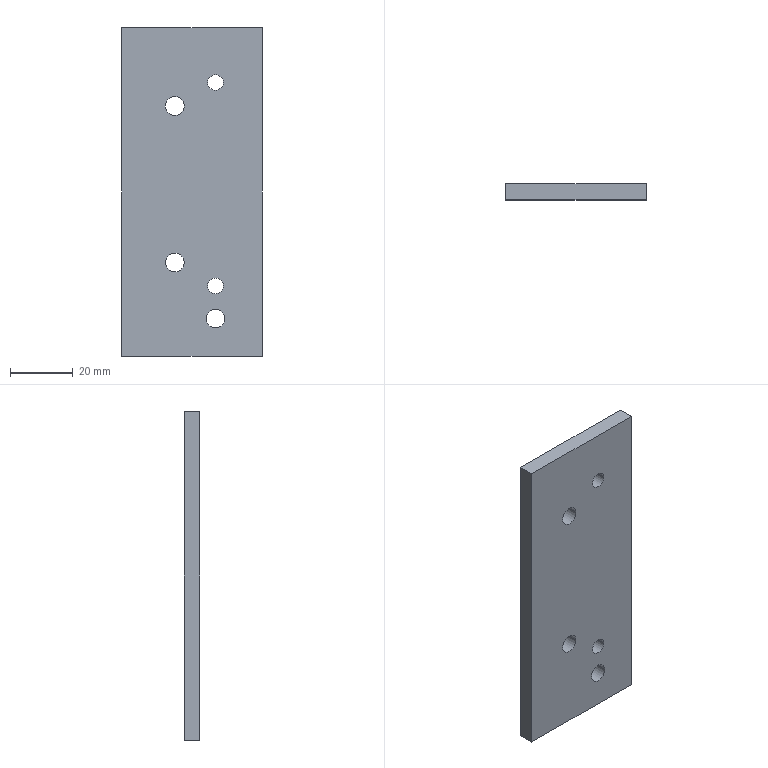Part | STEP file | 1 solid | 16 faces | box 45 x 5 x 105 mm | volume 23005 mm3 | cylinder 10 | plane 6 | commonest cylinder face diameters 6 x6 5 x4
STEP:
#1=CARTESIAN_POINT('',(0.,0.,0.));
#2=DIRECTION('',(0.,0.,1.));
#3=DIRECTION('',(1.,0.,0.));
#4=AXIS2_PLACEMENT_3D('',#1,#2,#3);
#5=CARTESIAN_POINT('',(10.,0.,-30.));
#6=VERTEX_POINT('',#5);
#7=CARTESIAN_POINT('',(10.,5.,-30.));
#8=VERTEX_POINT('',#7);
#9=CARTESIAN_POINT('',(10.,5.,-30.));
#10=DIRECTION('',(0.,1.,0.));
#11=VECTOR('',#10,1.);
#12=LINE('',#9,#11);
#13=CARTESIAN_POINT('',(7.5,5.,-30.));
#14=DIRECTION('',(0.,1.,0.));
#15=DIRECTION('',(1.,0.,0.));
#16=AXIS2_PLACEMENT_3D('',#13,#14,#15);
#17=CYLINDRICAL_SURFACE('',#16,2.5);
#18=CARTESIAN_POINT('',(6.283,0.));
#19=DIRECTION('',(0.,1.));
#20=VECTOR('',#19,1.);
#21=LINE('',#18,#20);
#22=(GEOMETRIC_REPRESENTATION_CONTEXT(2)PARAMETRIC_REPRESENTATION_CONTEXT()REPRESENTATION_CONTEXT('',''));
#23=DEFINITIONAL_REPRESENTATION('',(#21),#22);
#24=PCURVE('',#17,#23);
#25=CARTESIAN_POINT('',(7.5,5.,-30.));
#26=DIRECTION('',(0.,1.,0.));
#27=DIRECTION('',(1.,0.,0.));
#28=AXIS2_PLACEMENT_3D('',#25,#26,#27);
#29=CYLINDRICAL_SURFACE('',#28,2.5);
#30=CARTESIAN_POINT('',(0.,0.));
#31=DIRECTION('',(0.,1.));
#32=VECTOR('',#31,1.);
#33=LINE('',#30,#32);
#34=(GEOMETRIC_REPRESENTATION_CONTEXT(2)PARAMETRIC_REPRESENTATION_CONTEXT()REPRESENTATION_CONTEXT('',''));
#35=DEFINITIONAL_REPRESENTATION('',(#33),#34);
#36=PCURVE('',#29,#35);
#37=SURFACE_CURVE('',#12,(#24,#36),.PCURVE_S1.);
#38=EDGE_CURVE('',#6,#8,#37,.T.);
#39=ORIENTED_EDGE('',*,*,#38,.T.);
#40=CARTESIAN_POINT('',(5.,5.,-30.));
#41=VERTEX_POINT('',#40);
#42=CARTESIAN_POINT('',(7.5,5.,-30.));
#43=DIRECTION('',(0.,1.,0.));
#44=DIRECTION('',(1.,0.,0.));
#45=AXIS2_PLACEMENT_3D('',#42,#43,#44);
#46=CIRCLE('',#45,2.5);
#47=CARTESIAN_POINT('',(0.,0.));
#48=DIRECTION('',(1.,0.));
#49=VECTOR('',#48,1.);
#50=LINE('',#47,#49);
#51=(GEOMETRIC_REPRESENTATION_CONTEXT(2)PARAMETRIC_REPRESENTATION_CONTEXT()REPRESENTATION_CONTEXT('',''));
#52=DEFINITIONAL_REPRESENTATION('',(#50),#51);
#53=PCURVE('',#17,#52);
#54=CARTESIAN_POINT('',(0.,5.,0.));
#55=DIRECTION('',(0.,1.,0.));
#56=DIRECTION('',(0.,0.,1.));
#57=AXIS2_PLACEMENT_3D('',#54,#55,#56);
#58=PLANE('',#57);
#59=CARTESIAN_POINT('',(-30.,7.5));
#60=DIRECTION('',(0.,1.));
#61=AXIS2_PLACEMENT_2D('',#59,#60);
#62=CIRCLE('',#61,2.5);
#63=(GEOMETRIC_REPRESENTATION_CONTEXT(2)PARAMETRIC_REPRESENTATION_CONTEXT()REPRESENTATION_CONTEXT('',''));
#64=DEFINITIONAL_REPRESENTATION('',(#62),#63);
#65=PCURVE('',#58,#64);
#66=SURFACE_CURVE('',#46,(#53,#65),.PCURVE_S1.);
#67=EDGE_CURVE('',#41,#8,#66,.T.);
#68=ORIENTED_EDGE('',*,*,#67,.F.);
#69=CARTESIAN_POINT('',(5.,0.,-30.));
#70=VERTEX_POINT('',#69);
#71=CARTESIAN_POINT('',(5.,5.,-30.));
#72=DIRECTION('',(0.,1.,0.));
#73=VECTOR('',#72,1.);
#74=LINE('',#71,#73);
#75=CARTESIAN_POINT('',(3.142,0.));
#76=DIRECTION('',(0.,1.));
#77=VECTOR('',#76,1.);
#78=LINE('',#75,#77);
#79=(GEOMETRIC_REPRESENTATION_CONTEXT(2)PARAMETRIC_REPRESENTATION_CONTEXT()REPRESENTATION_CONTEXT('',''));
#80=DEFINITIONAL_REPRESENTATION('',(#78),#79);
#81=PCURVE('',#17,#80);
#82=CARTESIAN_POINT('',(3.142,0.));
#83=DIRECTION('',(0.,1.));
#84=VECTOR('',#83,1.);
#85=LINE('',#82,#84);
#86=(GEOMETRIC_REPRESENTATION_CONTEXT(2)PARAMETRIC_REPRESENTATION_CONTEXT()REPRESENTATION_CONTEXT('',''));
#87=DEFINITIONAL_REPRESENTATION('',(#85),#86);
#88=PCURVE('',#29,#87);
#89=SURFACE_CURVE('',#74,(#81,#88),.PCURVE_S1.);
#90=EDGE_CURVE('',#70,#41,#89,.T.);
#91=ORIENTED_EDGE('',*,*,#90,.F.);
#92=CARTESIAN_POINT('',(7.5,0.,-30.));
#93=DIRECTION('',(0.,1.,0.));
#94=DIRECTION('',(0.,0.,1.));
#95=AXIS2_PLACEMENT_3D('',#92,#93,#94);
#96=CIRCLE('',#95,2.5);
#97=CARTESIAN_POINT('',(-1.571,-5.));
#98=DIRECTION('',(1.,0.));
#99=VECTOR('',#98,1.);
#100=LINE('',#97,#99);
#101=(GEOMETRIC_REPRESENTATION_CONTEXT(2)PARAMETRIC_REPRESENTATION_CONTEXT()REPRESENTATION_CONTEXT('',''));
#102=DEFINITIONAL_REPRESENTATION('',(#100),#101);
#103=PCURVE('',#17,#102);
#104=CARTESIAN_POINT('',(0.,0.,0.));
#105=DIRECTION('',(0.,1.,0.));
#106=DIRECTION('',(0.,0.,1.));
#107=AXIS2_PLACEMENT_3D('',#104,#105,#106);
#108=PLANE('',#107);
#109=CARTESIAN_POINT('',(-30.,7.5));
#110=DIRECTION('',(1.,0.));
#111=AXIS2_PLACEMENT_2D('',#109,#110);
#112=CIRCLE('',#111,2.5);
#113=(GEOMETRIC_REPRESENTATION_CONTEXT(2)PARAMETRIC_REPRESENTATION_CONTEXT()REPRESENTATION_CONTEXT('',''));
#114=DEFINITIONAL_REPRESENTATION('',(#112),#113);
#115=PCURVE('',#108,#114);
#116=SURFACE_CURVE('',#96,(#103,#115),.PCURVE_S1.);
#117=EDGE_CURVE('',#70,#6,#116,.T.);
#118=ORIENTED_EDGE('',*,*,#117,.T.);
#119=EDGE_LOOP('',(#39,#68,#91,#118));
#120=FACE_BOUND('',#119,.F.);
#121=ADVANCED_FACE('',(#120),#17,.F.);
#122=CARTESIAN_POINT('',(10.,0.,35.));
#123=VERTEX_POINT('',#122);
#124=CARTESIAN_POINT('',(10.,5.,35.));
#125=VERTEX_POINT('',#124);
#126=CARTESIAN_POINT('',(10.,5.,35.));
#127=DIRECTION('',(0.,1.,0.));
#128=VECTOR('',#127,1.);
#129=LINE('',#126,#128);
#130=CARTESIAN_POINT('',(7.5,5.,35.));
#131=DIRECTION('',(0.,1.,0.));
#132=DIRECTION('',(1.,0.,0.));
#133=AXIS2_PLACEMENT_3D('',#130,#131,#132);
#134=CYLINDRICAL_SURFACE('',#133,2.5);
#135=CARTESIAN_POINT('',(6.283,0.));
#136=DIRECTION('',(0.,1.));
#137=VECTOR('',#136,1.);
#138=LINE('',#135,#137);
#139=(GEOMETRIC_REPRESENTATION_CONTEXT(2)PARAMETRIC_REPRESENTATION_CONTEXT()REPRESENTATION_CONTEXT('',''));
#140=DEFINITIONAL_REPRESENTATION('',(#138),#139);
#141=PCURVE('',#134,#140);
#142=CARTESIAN_POINT('',(7.5,5.,35.));
#143=DIRECTION('',(0.,1.,0.));
#144=DIRECTION('',(1.,0.,0.));
#145=AXIS2_PLACEMENT_3D('',#142,#143,#144);
#146=CYLINDRICAL_SURFACE('',#145,2.5);
#147=CARTESIAN_POINT('',(0.,0.));
#148=DIRECTION('',(0.,1.));
#149=VECTOR('',#148,1.);
#150=LINE('',#147,#149);
#151=(GEOMETRIC_REPRESENTATION_CONTEXT(2)PARAMETRIC_REPRESENTATION_CONTEXT()REPRESENTATION_CONTEXT('',''));
#152=DEFINITIONAL_REPRESENTATION('',(#150),#151);
#153=PCURVE('',#146,#152);
#154=SURFACE_CURVE('',#129,(#141,#153),.PCURVE_S1.);
#155=EDGE_CURVE('',#123,#125,#154,.T.);
#156=ORIENTED_EDGE('',*,*,#155,.T.);
#157=CARTESIAN_POINT('',(5.,5.,35.));
#158=VERTEX_POINT('',#157);
#159=CARTESIAN_POINT('',(7.5,5.,35.));
#160=DIRECTION('',(0.,1.,0.));
#161=DIRECTION('',(1.,0.,0.));
#162=AXIS2_PLACEMENT_3D('',#159,#160,#161);
#163=CIRCLE('',#162,2.5);
#164=CARTESIAN_POINT('',(0.,0.));
#165=DIRECTION('',(1.,0.));
#166=VECTOR('',#165,1.);
#167=LINE('',#164,#166);
#168=(GEOMETRIC_REPRESENTATION_CONTEXT(2)PARAMETRIC_REPRESENTATION_CONTEXT()REPRESENTATION_CONTEXT('',''));
#169=DEFINITIONAL_REPRESENTATION('',(#167),#168);
#170=PCURVE('',#134,#169);
#171=CARTESIAN_POINT('',(35.,7.5));
#172=DIRECTION('',(0.,1.));
#173=AXIS2_PLACEMENT_2D('',#171,#172);
#174=CIRCLE('',#173,2.5);
#175=(GEOMETRIC_REPRESENTATION_CONTEXT(2)PARAMETRIC_REPRESENTATION_CONTEXT()REPRESENTATION_CONTEXT('',''));
#176=DEFINITIONAL_REPRESENTATION('',(#174),#175);
#177=PCURVE('',#58,#176);
#178=SURFACE_CURVE('',#163,(#170,#177),.PCURVE_S1.);
#179=EDGE_CURVE('',#158,#125,#178,.T.);
#180=ORIENTED_EDGE('',*,*,#179,.F.);
#181=CARTESIAN_POINT('',(5.,0.,35.));
#182=VERTEX_POINT('',#181);
#183=CARTESIAN_POINT('',(5.,5.,35.));
#184=DIRECTION('',(0.,1.,0.));
#185=VECTOR('',#184,1.);
#186=LINE('',#183,#185);
#187=CARTESIAN_POINT('',(3.142,0.));
#188=DIRECTION('',(0.,1.));
#189=VECTOR('',#188,1.);
#190=LINE('',#187,#189);
#191=(GEOMETRIC_REPRESENTATION_CONTEXT(2)PARAMETRIC_REPRESENTATION_CONTEXT()REPRESENTATION_CONTEXT('',''));
#192=DEFINITIONAL_REPRESENTATION('',(#190),#191);
#193=PCURVE('',#134,#192);
#194=CARTESIAN_POINT('',(3.142,0.));
#195=DIRECTION('',(0.,1.));
#196=VECTOR('',#195,1.);
#197=LINE('',#194,#196);
#198=(GEOMETRIC_REPRESENTATION_CONTEXT(2)PARAMETRIC_REPRESENTATION_CONTEXT()REPRESENTATION_CONTEXT('',''));
#199=DEFINITIONAL_REPRESENTATION('',(#197),#198);
#200=PCURVE('',#146,#199);
#201=SURFACE_CURVE('',#186,(#193,#200),.PCURVE_S1.);
#202=EDGE_CURVE('',#182,#158,#201,.T.);
#203=ORIENTED_EDGE('',*,*,#202,.F.);
#204=CARTESIAN_POINT('',(7.5,0.,35.));
#205=DIRECTION('',(0.,1.,0.));
#206=DIRECTION('',(0.,0.,1.));
#207=AXIS2_PLACEMENT_3D('',#204,#205,#206);
#208=CIRCLE('',#207,2.5);
#209=CARTESIAN_POINT('',(-1.571,-5.));
#210=DIRECTION('',(1.,0.));
#211=VECTOR('',#210,1.);
#212=LINE('',#209,#211);
#213=(GEOMETRIC_REPRESENTATION_CONTEXT(2)PARAMETRIC_REPRESENTATION_CONTEXT()REPRESENTATION_CONTEXT('',''));
#214=DEFINITIONAL_REPRESENTATION('',(#212),#213);
#215=PCURVE('',#134,#214);
#216=CARTESIAN_POINT('',(35.,7.5));
#217=DIRECTION('',(1.,0.));
#218=AXIS2_PLACEMENT_2D('',#216,#217);
#219=CIRCLE('',#218,2.5);
#220=(GEOMETRIC_REPRESENTATION_CONTEXT(2)PARAMETRIC_REPRESENTATION_CONTEXT()REPRESENTATION_CONTEXT('',''));
#221=DEFINITIONAL_REPRESENTATION('',(#219),#220);
#222=PCURVE('',#108,#221);
#223=SURFACE_CURVE('',#208,(#215,#222),.PCURVE_S1.);
#224=EDGE_CURVE('',#182,#123,#223,.T.);
#225=ORIENTED_EDGE('',*,*,#224,.T.);
#226=EDGE_LOOP('',(#156,#180,#203,#225));
#227=FACE_BOUND('',#226,.F.);
#228=ADVANCED_FACE('',(#227),#134,.F.);
#229=CARTESIAN_POINT('',(-2.5,0.,27.5));
#230=VERTEX_POINT('',#229);
#231=CARTESIAN_POINT('',(-2.5,5.,27.5));
#232=VERTEX_POINT('',#231);
#233=CARTESIAN_POINT('',(-2.5,5.,27.5));
#234=DIRECTION('',(0.,1.,0.));
#235=VECTOR('',#234,1.);
#236=LINE('',#233,#235);
#237=CARTESIAN_POINT('',(-5.5,5.,27.5));
#238=DIRECTION('',(0.,1.,0.));
#239=DIRECTION('',(1.,0.,0.));
#240=AXIS2_PLACEMENT_3D('',#237,#238,#239);
#241=CYLINDRICAL_SURFACE('',#240,3.);
#242=CARTESIAN_POINT('',(6.283,0.));
#243=DIRECTION('',(0.,1.));
#244=VECTOR('',#243,1.);
#245=LINE('',#242,#244);
#246=(GEOMETRIC_REPRESENTATION_CONTEXT(2)PARAMETRIC_REPRESENTATION_CONTEXT()REPRESENTATION_CONTEXT('',''));
#247=DEFINITIONAL_REPRESENTATION('',(#245),#246);
#248=PCURVE('',#241,#247);
#249=CARTESIAN_POINT('',(-5.5,5.,27.5));
#250=DIRECTION('',(0.,1.,0.));
#251=DIRECTION('',(1.,0.,0.));
#252=AXIS2_PLACEMENT_3D('',#249,#250,#251);
#253=CYLINDRICAL_SURFACE('',#252,3.);
#254=CARTESIAN_POINT('',(0.,0.));
#255=DIRECTION('',(0.,1.));
#256=VECTOR('',#255,1.);
#257=LINE('',#254,#256);
#258=(GEOMETRIC_REPRESENTATION_CONTEXT(2)PARAMETRIC_REPRESENTATION_CONTEXT()REPRESENTATION_CONTEXT('',''));
#259=DEFINITIONAL_REPRESENTATION('',(#257),#258);
#260=PCURVE('',#253,#259);
#261=SURFACE_CURVE('',#236,(#248,#260),.PCURVE_S1.);
#262=EDGE_CURVE('',#230,#232,#261,.T.);
#263=ORIENTED_EDGE('',*,*,#262,.T.);
#264=CARTESIAN_POINT('',(-8.5,5.,27.5));
#265=VERTEX_POINT('',#264);
#266=CARTESIAN_POINT('',(-5.5,5.,27.5));
#267=DIRECTION('',(0.,1.,0.));
#268=DIRECTION('',(1.,0.,0.));
#269=AXIS2_PLACEMENT_3D('',#266,#267,#268);
#270=CIRCLE('',#269,3.);
#271=CARTESIAN_POINT('',(0.,0.));
#272=DIRECTION('',(1.,0.));
#273=VECTOR('',#272,1.);
#274=LINE('',#271,#273);
#275=(GEOMETRIC_REPRESENTATION_CONTEXT(2)PARAMETRIC_REPRESENTATION_CONTEXT()REPRESENTATION_CONTEXT('',''));
#276=DEFINITIONAL_REPRESENTATION('',(#274),#275);
#277=PCURVE('',#241,#276);
#278=CARTESIAN_POINT('',(27.5,-5.5));
#279=DIRECTION('',(0.,1.));
#280=AXIS2_PLACEMENT_2D('',#278,#279);
#281=CIRCLE('',#280,3.);
#282=(GEOMETRIC_REPRESENTATION_CONTEXT(2)PARAMETRIC_REPRESENTATION_CONTEXT()REPRESENTATION_CONTEXT('',''));
#283=DEFINITIONAL_REPRESENTATION('',(#281),#282);
#284=PCURVE('',#58,#283);
#285=SURFACE_CURVE('',#270,(#277,#284),.PCURVE_S1.);
#286=EDGE_CURVE('',#265,#232,#285,.T.);
#287=ORIENTED_EDGE('',*,*,#286,.F.);
#288=CARTESIAN_POINT('',(-8.5,0.,27.5));
#289=VERTEX_POINT('',#288);
#290=CARTESIAN_POINT('',(-8.5,5.,27.5));
#291=DIRECTION('',(0.,1.,0.));
#292=VECTOR('',#291,1.);
#293=LINE('',#290,#292);
#294=CARTESIAN_POINT('',(3.142,0.));
#295=DIRECTION('',(0.,1.));
#296=VECTOR('',#295,1.);
#297=LINE('',#294,#296);
#298=(GEOMETRIC_REPRESENTATION_CONTEXT(2)PARAMETRIC_REPRESENTATION_CONTEXT()REPRESENTATION_CONTEXT('',''));
#299=DEFINITIONAL_REPRESENTATION('',(#297),#298);
#300=PCURVE('',#241,#299);
#301=CARTESIAN_POINT('',(3.142,0.));
#302=DIRECTION('',(0.,1.));
#303=VECTOR('',#302,1.);
#304=LINE('',#301,#303);
#305=(GEOMETRIC_REPRESENTATION_CONTEXT(2)PARAMETRIC_REPRESENTATION_CONTEXT()REPRESENTATION_CONTEXT('',''));
#306=DEFINITIONAL_REPRESENTATION('',(#304),#305);
#307=PCURVE('',#253,#306);
#308=SURFACE_CURVE('',#293,(#300,#307),.PCURVE_S1.);
#309=EDGE_CURVE('',#289,#265,#308,.T.);
#310=ORIENTED_EDGE('',*,*,#309,.F.);
#311=CARTESIAN_POINT('',(-5.5,0.,27.5));
#312=DIRECTION('',(0.,1.,0.));
#313=DIRECTION('',(0.,0.,1.));
#314=AXIS2_PLACEMENT_3D('',#311,#312,#313);
#315=CIRCLE('',#314,3.);
#316=CARTESIAN_POINT('',(-1.571,-5.));
#317=DIRECTION('',(1.,0.));
#318=VECTOR('',#317,1.);
#319=LINE('',#316,#318);
#320=(GEOMETRIC_REPRESENTATION_CONTEXT(2)PARAMETRIC_REPRESENTATION_CONTEXT()REPRESENTATION_CONTEXT('',''));
#321=DEFINITIONAL_REPRESENTATION('',(#319),#320);
#322=PCURVE('',#241,#321);
#323=CARTESIAN_POINT('',(27.5,-5.5));
#324=DIRECTION('',(1.,0.));
#325=AXIS2_PLACEMENT_2D('',#323,#324);
#326=CIRCLE('',#325,3.);
#327=(GEOMETRIC_REPRESENTATION_CONTEXT(2)PARAMETRIC_REPRESENTATION_CONTEXT()REPRESENTATION_CONTEXT('',''));
#328=DEFINITIONAL_REPRESENTATION('',(#326),#327);
#329=PCURVE('',#108,#328);
#330=SURFACE_CURVE('',#315,(#322,#329),.PCURVE_S1.);
#331=EDGE_CURVE('',#289,#230,#330,.T.);
#332=ORIENTED_EDGE('',*,*,#331,.T.);
#333=EDGE_LOOP('',(#263,#287,#310,#332));
#334=FACE_BOUND('',#333,.F.);
#335=ADVANCED_FACE('',(#334),#241,.F.);
#336=CARTESIAN_POINT('',(-2.5,0.,-22.5));
#337=VERTEX_POINT('',#336);
#338=CARTESIAN_POINT('',(-2.5,5.,-22.5));
#339=VERTEX_POINT('',#338);
#340=CARTESIAN_POINT('',(-2.5,5.,-22.5));
#341=DIRECTION('',(0.,1.,0.));
#342=VECTOR('',#341,1.);
#343=LINE('',#340,#342);
#344=CARTESIAN_POINT('',(-5.5,5.,-22.5));
#345=DIRECTION('',(0.,1.,0.));
#346=DIRECTION('',(1.,0.,0.));
#347=AXIS2_PLACEMENT_3D('',#344,#345,#346);
#348=CYLINDRICAL_SURFACE('',#347,3.);
#349=CARTESIAN_POINT('',(6.283,0.));
#350=DIRECTION('',(0.,1.));
#351=VECTOR('',#350,1.);
#352=LINE('',#349,#351);
#353=(GEOMETRIC_REPRESENTATION_CONTEXT(2)PARAMETRIC_REPRESENTATION_CONTEXT()REPRESENTATION_CONTEXT('',''));
#354=DEFINITIONAL_REPRESENTATION('',(#352),#353);
#355=PCURVE('',#348,#354);
#356=CARTESIAN_POINT('',(-5.5,5.,-22.5));
#357=DIRECTION('',(0.,1.,0.));
#358=DIRECTION('',(1.,0.,0.));
#359=AXIS2_PLACEMENT_3D('',#356,#357,#358);
#360=CYLINDRICAL_SURFACE('',#359,3.);
#361=CARTESIAN_POINT('',(0.,0.));
#362=DIRECTION('',(0.,1.));
#363=VECTOR('',#362,1.);
#364=LINE('',#361,#363);
#365=(GEOMETRIC_REPRESENTATION_CONTEXT(2)PARAMETRIC_REPRESENTATION_CONTEXT()REPRESENTATION_CONTEXT('',''));
#366=DEFINITIONAL_REPRESENTATION('',(#364),#365);
#367=PCURVE('',#360,#366);
#368=SURFACE_CURVE('',#343,(#355,#367),.PCURVE_S1.);
#369=EDGE_CURVE('',#337,#339,#368,.T.);
#370=ORIENTED_EDGE('',*,*,#369,.T.);
#371=CARTESIAN_POINT('',(-8.5,5.,-22.5));
#372=VERTEX_POINT('',#371);
#373=CARTESIAN_POINT('',(-5.5,5.,-22.5));
#374=DIRECTION('',(0.,1.,0.));
#375=DIRECTION('',(1.,0.,0.));
#376=AXIS2_PLACEMENT_3D('',#373,#374,#375);
#377=CIRCLE('',#376,3.);
#378=CARTESIAN_POINT('',(0.,0.));
#379=DIRECTION('',(1.,0.));
#380=VECTOR('',#379,1.);
#381=LINE('',#378,#380);
#382=(GEOMETRIC_REPRESENTATION_CONTEXT(2)PARAMETRIC_REPRESENTATION_CONTEXT()REPRESENTATION_CONTEXT('',''));
#383=DEFINITIONAL_REPRESENTATION('',(#381),#382);
#384=PCURVE('',#348,#383);
#385=CARTESIAN_POINT('',(-22.5,-5.5));
#386=DIRECTION('',(0.,1.));
#387=AXIS2_PLACEMENT_2D('',#385,#386);
#388=CIRCLE('',#387,3.);
#389=(GEOMETRIC_REPRESENTATION_CONTEXT(2)PARAMETRIC_REPRESENTATION_CONTEXT()REPRESENTATION_CONTEXT('',''));
#390=DEFINITIONAL_REPRESENTATION('',(#388),#389);
#391=PCURVE('',#58,#390);
#392=SURFACE_CURVE('',#377,(#384,#391),.PCURVE_S1.);
#393=EDGE_CURVE('',#372,#339,#392,.T.);
#394=ORIENTED_EDGE('',*,*,#393,.F.);
#395=CARTESIAN_POINT('',(-8.5,0.,-22.5));
#396=VERTEX_POINT('',#395);
#397=CARTESIAN_POINT('',(-8.5,5.,-22.5));
#398=DIRECTION('',(0.,1.,0.));
#399=VECTOR('',#398,1.);
#400=LINE('',#397,#399);
#401=CARTESIAN_POINT('',(3.142,0.));
#402=DIRECTION('',(0.,1.));
#403=VECTOR('',#402,1.);
#404=LINE('',#401,#403);
#405=(GEOMETRIC_REPRESENTATION_CONTEXT(2)PARAMETRIC_REPRESENTATION_CONTEXT()REPRESENTATION_CONTEXT('',''));
#406=DEFINITIONAL_REPRESENTATION('',(#404),#405);
#407=PCURVE('',#348,#406);
#408=CARTESIAN_POINT('',(3.142,0.));
#409=DIRECTION('',(0.,1.));
#410=VECTOR('',#409,1.);
#411=LINE('',#408,#410);
#412=(GEOMETRIC_REPRESENTATION_CONTEXT(2)PARAMETRIC_REPRESENTATION_CONTEXT()REPRESENTATION_CONTEXT('',''));
#413=DEFINITIONAL_REPRESENTATION('',(#411),#412);
#414=PCURVE('',#360,#413);
#415=SURFACE_CURVE('',#400,(#407,#414),.PCURVE_S1.);
#416=EDGE_CURVE('',#396,#372,#415,.T.);
#417=ORIENTED_EDGE('',*,*,#416,.F.);
#418=CARTESIAN_POINT('',(-5.5,0.,-22.5));
#419=DIRECTION('',(0.,1.,0.));
#420=DIRECTION('',(0.,0.,1.));
#421=AXIS2_PLACEMENT_3D('',#418,#419,#420);
#422=CIRCLE('',#421,3.);
#423=CARTESIAN_POINT('',(-1.571,-5.));
#424=DIRECTION('',(1.,0.));
#425=VECTOR('',#424,1.);
#426=LINE('',#423,#425);
#427=(GEOMETRIC_REPRESENTATION_CONTEXT(2)PARAMETRIC_REPRESENTATION_CONTEXT()REPRESENTATION_CONTEXT('',''));
#428=DEFINITIONAL_REPRESENTATION('',(#426),#427);
#429=PCURVE('',#348,#428);
#430=CARTESIAN_POINT('',(-22.5,-5.5));
#431=DIRECTION('',(1.,0.));
#432=AXIS2_PLACEMENT_2D('',#430,#431);
#433=CIRCLE('',#432,3.);
#434=(GEOMETRIC_REPRESENTATION_CONTEXT(2)PARAMETRIC_REPRESENTATION_CONTEXT()REPRESENTATION_CONTEXT('',''));
#435=DEFINITIONAL_REPRESENTATION('',(#433),#434);
#436=PCURVE('',#108,#435);
#437=SURFACE_CURVE('',#422,(#429,#436),.PCURVE_S1.);
#438=EDGE_CURVE('',#396,#337,#437,.T.);
#439=ORIENTED_EDGE('',*,*,#438,.T.);
#440=EDGE_LOOP('',(#370,#394,#417,#439));
#441=FACE_BOUND('',#440,.F.);
#442=ADVANCED_FACE('',(#441),#348,.F.);
#443=CARTESIAN_POINT('',(10.5,0.,-40.5));
#444=VERTEX_POINT('',#443);
#445=CARTESIAN_POINT('',(10.5,5.,-40.5));
#446=VERTEX_POINT('',#445);
#447=CARTESIAN_POINT('',(10.5,5.,-40.5));
#448=DIRECTION('',(0.,1.,0.));
#449=VECTOR('',#448,1.);
#450=LINE('',#447,#449);
#451=CARTESIAN_POINT('',(7.5,5.,-40.5));
#452=DIRECTION('',(0.,1.,0.));
#453=DIRECTION('',(1.,0.,0.));
#454=AXIS2_PLACEMENT_3D('',#451,#452,#453);
#455=CYLINDRICAL_SURFACE('',#454,3.);
#456=CARTESIAN_POINT('',(6.283,0.));
#457=DIRECTION('',(0.,1.));
#458=VECTOR('',#457,1.);
#459=LINE('',#456,#458);
#460=(GEOMETRIC_REPRESENTATION_CONTEXT(2)PARAMETRIC_REPRESENTATION_CONTEXT()REPRESENTATION_CONTEXT('',''));
#461=DEFINITIONAL_REPRESENTATION('',(#459),#460);
#462=PCURVE('',#455,#461);
#463=CARTESIAN_POINT('',(7.5,5.,-40.5));
#464=DIRECTION('',(0.,1.,0.));
#465=DIRECTION('',(1.,0.,0.));
#466=AXIS2_PLACEMENT_3D('',#463,#464,#465);
#467=CYLINDRICAL_SURFACE('',#466,3.);
#468=CARTESIAN_POINT('',(0.,0.));
#469=DIRECTION('',(0.,1.));
#470=VECTOR('',#469,1.);
#471=LINE('',#468,#470);
#472=(GEOMETRIC_REPRESENTATION_CONTEXT(2)PARAMETRIC_REPRESENTATION_CONTEXT()REPRESENTATION_CONTEXT('',''));
#473=DEFINITIONAL_REPRESENTATION('',(#471),#472);
#474=PCURVE('',#467,#473);
#475=SURFACE_CURVE('',#450,(#462,#474),.PCURVE_S1.);
#476=EDGE_CURVE('',#444,#446,#475,.T.);
#477=ORIENTED_EDGE('',*,*,#476,.T.);
#478=CARTESIAN_POINT('',(4.5,5.,-40.5));
#479=VERTEX_POINT('',#478);
#480=CARTESIAN_POINT('',(7.5,5.,-40.5));
#481=DIRECTION('',(0.,1.,0.));
#482=DIRECTION('',(1.,0.,0.));
#483=AXIS2_PLACEMENT_3D('',#480,#481,#482);
#484=CIRCLE('',#483,3.);
#485=CARTESIAN_POINT('',(0.,0.));
#486=DIRECTION('',(1.,0.));
#487=VECTOR('',#486,1.);
#488=LINE('',#485,#487);
#489=(GEOMETRIC_REPRESENTATION_CONTEXT(2)PARAMETRIC_REPRESENTATION_CONTEXT()REPRESENTATION_CONTEXT('',''));
#490=DEFINITIONAL_REPRESENTATION('',(#488),#489);
#491=PCURVE('',#455,#490);
#492=CARTESIAN_POINT('',(-40.5,7.5));
#493=DIRECTION('',(0.,1.));
#494=AXIS2_PLACEMENT_2D('',#492,#493);
#495=CIRCLE('',#494,3.);
#496=(GEOMETRIC_REPRESENTATION_CONTEXT(2)PARAMETRIC_REPRESENTATION_CONTEXT()REPRESENTATION_CONTEXT('',''));
#497=DEFINITIONAL_REPRESENTATION('',(#495),#496);
#498=PCURVE('',#58,#497);
#499=SURFACE_CURVE('',#484,(#491,#498),.PCURVE_S1.);
#500=EDGE_CURVE('',#479,#446,#499,.T.);
#501=ORIENTED_EDGE('',*,*,#500,.F.);
#502=CARTESIAN_POINT('',(4.5,0.,-40.5));
#503=VERTEX_POINT('',#502);
#504=CARTESIAN_POINT('',(4.5,5.,-40.5));
#505=DIRECTION('',(0.,1.,0.));
#506=VECTOR('',#505,1.);
#507=LINE('',#504,#506);
#508=CARTESIAN_POINT('',(3.142,0.));
#509=DIRECTION('',(0.,1.));
#510=VECTOR('',#509,1.);
#511=LINE('',#508,#510);
#512=(GEOMETRIC_REPRESENTATION_CONTEXT(2)PARAMETRIC_REPRESENTATION_CONTEXT()REPRESENTATION_CONTEXT('',''));
#513=DEFINITIONAL_REPRESENTATION('',(#511),#512);
#514=PCURVE('',#455,#513);
#515=CARTESIAN_POINT('',(3.142,0.));
#516=DIRECTION('',(0.,1.));
#517=VECTOR('',#516,1.);
#518=LINE('',#515,#517);
#519=(GEOMETRIC_REPRESENTATION_CONTEXT(2)PARAMETRIC_REPRESENTATION_CONTEXT()REPRESENTATION_CONTEXT('',''));
#520=DEFINITIONAL_REPRESENTATION('',(#518),#519);
#521=PCURVE('',#467,#520);
#522=SURFACE_CURVE('',#507,(#514,#521),.PCURVE_S1.);
#523=EDGE_CURVE('',#503,#479,#522,.T.);
#524=ORIENTED_EDGE('',*,*,#523,.F.);
#525=CARTESIAN_POINT('',(7.5,0.,-40.5));
#526=DIRECTION('',(0.,1.,0.));
#527=DIRECTION('',(0.,0.,1.));
#528=AXIS2_PLACEMENT_3D('',#525,#526,#527);
#529=CIRCLE('',#528,3.);
#530=CARTESIAN_POINT('',(-1.571,-5.));
#531=DIRECTION('',(1.,0.));
#532=VECTOR('',#531,1.);
#533=LINE('',#530,#532);
#534=(GEOMETRIC_REPRESENTATION_CONTEXT(2)PARAMETRIC_REPRESENTATION_CONTEXT()REPRESENTATION_CONTEXT('',''));
#535=DEFINITIONAL_REPRESENTATION('',(#533),#534);
#536=PCURVE('',#455,#535);
#537=CARTESIAN_POINT('',(-40.5,7.5));
#538=DIRECTION('',(1.,0.));
#539=AXIS2_PLACEMENT_2D('',#537,#538);
#540=CIRCLE('',#539,3.);
#541=(GEOMETRIC_REPRESENTATION_CONTEXT(2)PARAMETRIC_REPRESENTATION_CONTEXT()REPRESENTATION_CONTEXT('',''));
#542=DEFINITIONAL_REPRESENTATION('',(#540),#541);
#543=PCURVE('',#108,#542);
#544=SURFACE_CURVE('',#529,(#536,#543),.PCURVE_S1.);
#545=EDGE_CURVE('',#503,#444,#544,.T.);
#546=ORIENTED_EDGE('',*,*,#545,.T.);
#547=EDGE_LOOP('',(#477,#501,#524,#546));
#548=FACE_BOUND('',#547,.F.);
#549=ADVANCED_FACE('',(#548),#455,.F.);
#550=CARTESIAN_POINT('',(-22.5,0.,-52.5));
#551=VERTEX_POINT('',#550);
#552=CARTESIAN_POINT('',(-22.5,0.,52.5));
#553=VERTEX_POINT('',#552);
#554=CARTESIAN_POINT('',(-22.5,0.,52.5));
#555=DIRECTION('',(0.,0.,1.));
#556=VECTOR('',#555,1.);
#557=LINE('',#554,#556);
#558=CARTESIAN_POINT('',(-22.5,5.,52.5));
#559=DIRECTION('',(1.,0.,0.));
#560=DIRECTION('',(0.,0.,-1.));
#561=AXIS2_PLACEMENT_3D('',#558,#559,#560);
#562=PLANE('',#561);
#563=CARTESIAN_POINT('',(0.,-5.));
#564=DIRECTION('',(-1.,0.));
#565=VECTOR('',#564,1.);
#566=LINE('',#563,#565);
#567=(GEOMETRIC_REPRESENTATION_CONTEXT(2)PARAMETRIC_REPRESENTATION_CONTEXT()REPRESENTATION_CONTEXT('',''));
#568=DEFINITIONAL_REPRESENTATION('',(#566),#567);
#569=PCURVE('',#562,#568);
#570=CARTESIAN_POINT('',(52.5,-22.5));
#571=DIRECTION('',(1.,0.));
#572=VECTOR('',#571,1.);
#573=LINE('',#570,#572);
#574=(GEOMETRIC_REPRESENTATION_CONTEXT(2)PARAMETRIC_REPRESENTATION_CONTEXT()REPRESENTATION_CONTEXT('',''));
#575=DEFINITIONAL_REPRESENTATION('',(#573),#574);
#576=PCURVE('',#108,#575);
#577=SURFACE_CURVE('',#557,(#569,#576),.PCURVE_S1.);
#578=EDGE_CURVE('',#551,#553,#577,.T.);
#579=ORIENTED_EDGE('',*,*,#578,.T.);
#580=CARTESIAN_POINT('',(-22.5,5.,52.5));
#581=VERTEX_POINT('',#580);
#582=CARTESIAN_POINT('',(-22.5,5.,52.5));
#583=DIRECTION('',(0.,-1.,0.));
#584=VECTOR('',#583,1.);
#585=LINE('',#582,#584);
#586=CARTESIAN_POINT('',(0.,0.));
#587=DIRECTION('',(0.,-1.));
#588=VECTOR('',#587,1.);
#589=LINE('',#586,#588);
#590=(GEOMETRIC_REPRESENTATION_CONTEXT(2)PARAMETRIC_REPRESENTATION_CONTEXT()REPRESENTATION_CONTEXT('',''));
#591=DEFINITIONAL_REPRESENTATION('',(#589),#590);
#592=PCURVE('',#562,#591);
#593=CARTESIAN_POINT('',(22.5,5.,52.5));
#594=DIRECTION('',(0.,0.,-1.));
#595=DIRECTION('',(-1.,0.,0.));
#596=AXIS2_PLACEMENT_3D('',#593,#594,#595);
#597=PLANE('',#596);
#598=CARTESIAN_POINT('',(45.,0.));
#599=DIRECTION('',(0.,-1.));
#600=VECTOR('',#599,1.);
#601=LINE('',#598,#600);
#602=(GEOMETRIC_REPRESENTATION_CONTEXT(2)PARAMETRIC_REPRESENTATION_CONTEXT()REPRESENTATION_CONTEXT('',''));
#603=DEFINITIONAL_REPRESENTATION('',(#601),#602);
#604=PCURVE('',#597,#603);
#605=SURFACE_CURVE('',#585,(#592,#604),.PCURVE_S1.);
#606=EDGE_CURVE('',#581,#553,#605,.T.);
#607=ORIENTED_EDGE('',*,*,#606,.F.);
#608=CARTESIAN_POINT('',(-22.5,5.,-52.5));
#609=VERTEX_POINT('',#608);
#610=CARTESIAN_POINT('',(-22.5,5.,52.5));
#611=DIRECTION('',(0.,0.,1.));
#612=VECTOR('',#611,1.);
#613=LINE('',#610,#612);
#614=CARTESIAN_POINT('',(0.,0.));
#615=DIRECTION('',(-1.,0.));
#616=VECTOR('',#615,1.);
#617=LINE('',#614,#616);
#618=(GEOMETRIC_REPRESENTATION_CONTEXT(2)PARAMETRIC_REPRESENTATION_CONTEXT()REPRESENTATION_CONTEXT('',''));
#619=DEFINITIONAL_REPRESENTATION('',(#617),#618);
#620=PCURVE('',#562,#619);
#621=CARTESIAN_POINT('',(52.5,-22.5));
#622=DIRECTION('',(1.,0.));
#623=VECTOR('',#622,1.);
#624=LINE('',#621,#623);
#625=(GEOMETRIC_REPRESENTATION_CONTEXT(2)PARAMETRIC_REPRESENTATION_CONTEXT()REPRESENTATION_CONTEXT('',''));
#626=DEFINITIONAL_REPRESENTATION('',(#624),#625);
#627=PCURVE('',#58,#626);
#628=SURFACE_CURVE('',#613,(#620,#627),.PCURVE_S1.);
#629=EDGE_CURVE('',#609,#581,#628,.T.);
#630=ORIENTED_EDGE('',*,*,#629,.F.);
#631=CARTESIAN_POINT('',(-22.5,5.,-52.5));
#632=DIRECTION('',(0.,-1.,0.));
#633=VECTOR('',#632,1.);
#634=LINE('',#631,#633);
#635=CARTESIAN_POINT('',(105.,0.));
#636=DIRECTION('',(0.,-1.));
#637=VECTOR('',#636,1.);
#638=LINE('',#635,#637);
#639=(GEOMETRIC_REPRESENTATION_CONTEXT(2)PARAMETRIC_REPRESENTATION_CONTEXT()REPRESENTATION_CONTEXT('',''));
#640=DEFINITIONAL_REPRESENTATION('',(#638),#639);
#641=PCURVE('',#562,#640);
#642=CARTESIAN_POINT('',(22.5,5.,-52.5));
#643=DIRECTION('',(0.,0.,1.));
#644=DIRECTION('',(1.,0.,0.));
#645=AXIS2_PLACEMENT_3D('',#642,#643,#644);
#646=PLANE('',#645);
#647=CARTESIAN_POINT('',(-45.,0.));
#648=DIRECTION('',(0.,-1.));
#649=VECTOR('',#648,1.);
#650=LINE('',#647,#649);
#651=(GEOMETRIC_REPRESENTATION_CONTEXT(2)PARAMETRIC_REPRESENTATION_CONTEXT()REPRESENTATION_CONTEXT('',''));
#652=DEFINITIONAL_REPRESENTATION('',(#650),#651);
#653=PCURVE('',#646,#652);
#654=SURFACE_CURVE('',#634,(#641,#653),.PCURVE_S1.);
#655=EDGE_CURVE('',#609,#551,#654,.T.);
#656=ORIENTED_EDGE('',*,*,#655,.T.);
#657=EDGE_LOOP('',(#579,#607,#630,#656));
#658=FACE_BOUND('',#657,.T.);
#659=ADVANCED_FACE('',(#658),#562,.F.);
#660=CARTESIAN_POINT('',(22.5,0.,52.5));
#661=VERTEX_POINT('',#660);
#662=CARTESIAN_POINT('',(22.5,0.,52.5));
#663=DIRECTION('',(1.,0.,0.));
#664=VECTOR('',#663,1.);
#665=LINE('',#662,#664);
#666=CARTESIAN_POINT('',(0.,-5.));
#667=DIRECTION('',(-1.,0.));
#668=VECTOR('',#667,1.);
#669=LINE('',#666,#668);
#670=(GEOMETRIC_REPRESENTATION_CONTEXT(2)PARAMETRIC_REPRESENTATION_CONTEXT()REPRESENTATION_CONTEXT('',''));
#671=DEFINITIONAL_REPRESENTATION('',(#669),#670);
#672=PCURVE('',#597,#671);
#673=CARTESIAN_POINT('',(52.5,22.5));
#674=DIRECTION('',(0.,1.));
#675=VECTOR('',#674,1.);
#676=LINE('',#673,#675);
#677=(GEOMETRIC_REPRESENTATION_CONTEXT(2)PARAMETRIC_REPRESENTATION_CONTEXT()REPRESENTATION_CONTEXT('',''));
#678=DEFINITIONAL_REPRESENTATION('',(#676),#677);
#679=PCURVE('',#108,#678);
#680=SURFACE_CURVE('',#665,(#672,#679),.PCURVE_S1.);
#681=EDGE_CURVE('',#553,#661,#680,.T.);
#682=ORIENTED_EDGE('',*,*,#681,.T.);
#683=CARTESIAN_POINT('',(22.5,5.,52.5));
#684=VERTEX_POINT('',#683);
#685=CARTESIAN_POINT('',(22.5,5.,52.5));
#686=DIRECTION('',(0.,-1.,0.));
#687=VECTOR('',#686,1.);
#688=LINE('',#685,#687);
#689=CARTESIAN_POINT('',(0.,0.));
#690=DIRECTION('',(0.,-1.));
#691=VECTOR('',#690,1.);
#692=LINE('',#689,#691);
#693=(GEOMETRIC_REPRESENTATION_CONTEXT(2)PARAMETRIC_REPRESENTATION_CONTEXT()REPRESENTATION_CONTEXT('',''));
#694=DEFINITIONAL_REPRESENTATION('',(#692),#693);
#695=PCURVE('',#597,#694);
#696=CARTESIAN_POINT('',(22.5,5.,52.5));
#697=DIRECTION('',(-1.,0.,0.));
#698=DIRECTION('',(0.,0.,1.));
#699=AXIS2_PLACEMENT_3D('',#696,#697,#698);
#700=PLANE('',#699);
#701=CARTESIAN_POINT('',(0.,0.));
#702=DIRECTION('',(0.,-1.));
#703=VECTOR('',#702,1.);
#704=LINE('',#701,#703);
#705=(GEOMETRIC_REPRESENTATION_CONTEXT(2)PARAMETRIC_REPRESENTATION_CONTEXT()REPRESENTATION_CONTEXT('',''));
#706=DEFINITIONAL_REPRESENTATION('',(#704),#705);
#707=PCURVE('',#700,#706);
#708=SURFACE_CURVE('',#688,(#695,#707),.PCURVE_S1.);
#709=EDGE_CURVE('',#684,#661,#708,.T.);
#710=ORIENTED_EDGE('',*,*,#709,.F.);
#711=CARTESIAN_POINT('',(22.5,5.,52.5));
#712=DIRECTION('',(1.,0.,0.));
#713=VECTOR('',#712,1.);
#714=LINE('',#711,#713);
#715=CARTESIAN_POINT('',(0.,0.));
#716=DIRECTION('',(-1.,0.));
#717=VECTOR('',#716,1.);
#718=LINE('',#715,#717);
#719=(GEOMETRIC_REPRESENTATION_CONTEXT(2)PARAMETRIC_REPRESENTATION_CONTEXT()REPRESENTATION_CONTEXT('',''));
#720=DEFINITIONAL_REPRESENTATION('',(#718),#719);
#721=PCURVE('',#597,#720);
#722=CARTESIAN_POINT('',(52.5,22.5));
#723=DIRECTION('',(0.,1.));
#724=VECTOR('',#723,1.);
#725=LINE('',#722,#724);
#726=(GEOMETRIC_REPRESENTATION_CONTEXT(2)PARAMETRIC_REPRESENTATION_CONTEXT()REPRESENTATION_CONTEXT('',''));
#727=DEFINITIONAL_REPRESENTATION('',(#725),#726);
#728=PCURVE('',#58,#727);
#729=SURFACE_CURVE('',#714,(#721,#728),.PCURVE_S1.);
#730=EDGE_CURVE('',#581,#684,#729,.T.);
#731=ORIENTED_EDGE('',*,*,#730,.F.);
#732=ORIENTED_EDGE('',*,*,#606,.T.);
#733=EDGE_LOOP('',(#682,#710,#731,#732));
#734=FACE_BOUND('',#733,.T.);
#735=ADVANCED_FACE('',(#734),#597,.F.);
#736=CARTESIAN_POINT('',(22.5,0.,-52.5));
#737=VERTEX_POINT('',#736);
#738=CARTESIAN_POINT('',(22.5,0.,52.5));
#739=DIRECTION('',(0.,0.,-1.));
#740=VECTOR('',#739,1.);
#741=LINE('',#738,#740);
#742=CARTESIAN_POINT('',(0.,-5.));
#743=DIRECTION('',(-1.,0.));
#744=VECTOR('',#743,1.);
#745=LINE('',#742,#744);
#746=(GEOMETRIC_REPRESENTATION_CONTEXT(2)PARAMETRIC_REPRESENTATION_CONTEXT()REPRESENTATION_CONTEXT('',''));
#747=DEFINITIONAL_REPRESENTATION('',(#745),#746);
#748=PCURVE('',#700,#747);
#749=CARTESIAN_POINT('',(52.5,22.5));
#750=DIRECTION('',(-1.,0.));
#751=VECTOR('',#750,1.);
#752=LINE('',#749,#751);
#753=(GEOMETRIC_REPRESENTATION_CONTEXT(2)PARAMETRIC_REPRESENTATION_CONTEXT()REPRESENTATION_CONTEXT('',''));
#754=DEFINITIONAL_REPRESENTATION('',(#752),#753);
#755=PCURVE('',#108,#754);
#756=SURFACE_CURVE('',#741,(#748,#755),.PCURVE_S1.);
#757=EDGE_CURVE('',#661,#737,#756,.T.);
#758=ORIENTED_EDGE('',*,*,#757,.T.);
#759=CARTESIAN_POINT('',(22.5,5.,-52.5));
#760=VERTEX_POINT('',#759);
#761=CARTESIAN_POINT('',(22.5,5.,-52.5));
#762=DIRECTION('',(0.,-1.,0.));
#763=VECTOR('',#762,1.);
#764=LINE('',#761,#763);
#765=CARTESIAN_POINT('',(-105.,0.));
#766=DIRECTION('',(0.,-1.));
#767=VECTOR('',#766,1.);
#768=LINE('',#765,#767);
#769=(GEOMETRIC_REPRESENTATION_CONTEXT(2)PARAMETRIC_REPRESENTATION_CONTEXT()REPRESENTATION_CONTEXT('',''));
#770=DEFINITIONAL_REPRESENTATION('',(#768),#769);
#771=PCURVE('',#700,#770);
#772=CARTESIAN_POINT('',(0.,0.));
#773=DIRECTION('',(0.,-1.));
#774=VECTOR('',#773,1.);
#775=LINE('',#772,#774);
#776=(GEOMETRIC_REPRESENTATION_CONTEXT(2)PARAMETRIC_REPRESENTATION_CONTEXT()REPRESENTATION_CONTEXT('',''));
#777=DEFINITIONAL_REPRESENTATION('',(#775),#776);
#778=PCURVE('',#646,#777);
#779=SURFACE_CURVE('',#764,(#771,#778),.PCURVE_S1.);
#780=EDGE_CURVE('',#760,#737,#779,.T.);
#781=ORIENTED_EDGE('',*,*,#780,.F.);
#782=CARTESIAN_POINT('',(22.5,5.,52.5));
#783=DIRECTION('',(0.,0.,-1.));
#784=VECTOR('',#783,1.);
#785=LINE('',#782,#784);
#786=CARTESIAN_POINT('',(0.,0.));
#787=DIRECTION('',(-1.,0.));
#788=VECTOR('',#787,1.);
#789=LINE('',#786,#788);
#790=(GEOMETRIC_REPRESENTATION_CONTEXT(2)PARAMETRIC_REPRESENTATION_CONTEXT()REPRESENTATION_CONTEXT('',''));
#791=DEFINITIONAL_REPRESENTATION('',(#789),#790);
#792=PCURVE('',#700,#791);
#793=CARTESIAN_POINT('',(52.5,22.5));
#794=DIRECTION('',(-1.,0.));
#795=VECTOR('',#794,1.);
#796=LINE('',#793,#795);
#797=(GEOMETRIC_REPRESENTATION_CONTEXT(2)PARAMETRIC_REPRESENTATION_CONTEXT()REPRESENTATION_CONTEXT('',''));
#798=DEFINITIONAL_REPRESENTATION('',(#796),#797);
#799=PCURVE('',#58,#798);
#800=SURFACE_CURVE('',#785,(#792,#799),.PCURVE_S1.);
#801=EDGE_CURVE('',#684,#760,#800,.T.);
#802=ORIENTED_EDGE('',*,*,#801,.F.);
#803=ORIENTED_EDGE('',*,*,#709,.T.);
#804=EDGE_LOOP('',(#758,#781,#802,#803));
#805=FACE_BOUND('',#804,.T.);
#806=ADVANCED_FACE('',(#805),#700,.F.);
#807=CARTESIAN_POINT('',(22.5,0.,-52.5));
#808=DIRECTION('',(-1.,0.,0.));
#809=VECTOR('',#808,1.);
#810=LINE('',#807,#809);
#811=CARTESIAN_POINT('',(0.,-5.));
#812=DIRECTION('',(-1.,0.));
#813=VECTOR('',#812,1.);
#814=LINE('',#811,#813);
#815=(GEOMETRIC_REPRESENTATION_CONTEXT(2)PARAMETRIC_REPRESENTATION_CONTEXT()REPRESENTATION_CONTEXT('',''));
#816=DEFINITIONAL_REPRESENTATION('',(#814),#815);
#817=PCURVE('',#646,#816);
#818=CARTESIAN_POINT('',(-52.5,22.5));
#819=DIRECTION('',(0.,-1.));
#820=VECTOR('',#819,1.);
#821=LINE('',#818,#820);
#822=(GEOMETRIC_REPRESENTATION_CONTEXT(2)PARAMETRIC_REPRESENTATION_CONTEXT()REPRESENTATION_CONTEXT('',''));
#823=DEFINITIONAL_REPRESENTATION('',(#821),#822);
#824=PCURVE('',#108,#823);
#825=SURFACE_CURVE('',#810,(#817,#824),.PCURVE_S1.);
#826=EDGE_CURVE('',#737,#551,#825,.T.);
#827=ORIENTED_EDGE('',*,*,#826,.T.);
#828=ORIENTED_EDGE('',*,*,#655,.F.);
#829=CARTESIAN_POINT('',(22.5,5.,-52.5));
#830=DIRECTION('',(-1.,0.,0.));
#831=VECTOR('',#830,1.);
#832=LINE('',#829,#831);
#833=CARTESIAN_POINT('',(0.,0.));
#834=DIRECTION('',(-1.,0.));
#835=VECTOR('',#834,1.);
#836=LINE('',#833,#835);
#837=(GEOMETRIC_REPRESENTATION_CONTEXT(2)PARAMETRIC_REPRESENTATION_CONTEXT()REPRESENTATION_CONTEXT('',''));
#838=DEFINITIONAL_REPRESENTATION('',(#836),#837);
#839=PCURVE('',#646,#838);
#840=CARTESIAN_POINT('',(-52.5,22.5));
#841=DIRECTION('',(0.,-1.));
#842=VECTOR('',#841,1.);
#843=LINE('',#840,#842);
#844=(GEOMETRIC_REPRESENTATION_CONTEXT(2)PARAMETRIC_REPRESENTATION_CONTEXT()REPRESENTATION_CONTEXT('',''));
#845=DEFINITIONAL_REPRESENTATION('',(#843),#844);
#846=PCURVE('',#58,#845);
#847=SURFACE_CURVE('',#832,(#839,#846),.PCURVE_S1.);
#848=EDGE_CURVE('',#760,#609,#847,.T.);
#849=ORIENTED_EDGE('',*,*,#848,.F.);
#850=ORIENTED_EDGE('',*,*,#780,.T.);
#851=EDGE_LOOP('',(#827,#828,#849,#850));
#852=FACE_BOUND('',#851,.T.);
#853=ADVANCED_FACE('',(#852),#646,.F.);
#854=CARTESIAN_POINT('',(7.5,5.,-30.));
#855=DIRECTION('',(0.,1.,0.));
#856=DIRECTION('',(1.,0.,0.));
#857=AXIS2_PLACEMENT_3D('',#854,#855,#856);
#858=CIRCLE('',#857,2.5);
#859=CARTESIAN_POINT('',(-30.,7.5));
#860=DIRECTION('',(0.,1.));
#861=AXIS2_PLACEMENT_2D('',#859,#860);
#862=CIRCLE('',#861,2.5);
#863=(GEOMETRIC_REPRESENTATION_CONTEXT(2)PARAMETRIC_REPRESENTATION_CONTEXT()REPRESENTATION_CONTEXT('',''));
#864=DEFINITIONAL_REPRESENTATION('',(#862),#863);
#865=PCURVE('',#58,#864);
#866=CARTESIAN_POINT('',(0.,0.));
#867=DIRECTION('',(1.,0.));
#868=VECTOR('',#867,1.);
#869=LINE('',#866,#868);
#870=(GEOMETRIC_REPRESENTATION_CONTEXT(2)PARAMETRIC_REPRESENTATION_CONTEXT()REPRESENTATION_CONTEXT('',''));
#871=DEFINITIONAL_REPRESENTATION('',(#869),#870);
#872=PCURVE('',#29,#871);
#873=SURFACE_CURVE('',#858,(#865,#872),.PCURVE_S1.);
#874=EDGE_CURVE('',#8,#41,#873,.T.);
#875=ORIENTED_EDGE('',*,*,#874,.F.);
#876=ORIENTED_EDGE('',*,*,#67,.F.);
#877=EDGE_LOOP('',(#875,#876));
#878=FACE_BOUND('',#877,.T.);
#879=CARTESIAN_POINT('',(7.5,5.,35.));
#880=DIRECTION('',(0.,1.,0.));
#881=DIRECTION('',(1.,0.,0.));
#882=AXIS2_PLACEMENT_3D('',#879,#880,#881);
#883=CIRCLE('',#882,2.5);
#884=CARTESIAN_POINT('',(35.,7.5));
#885=DIRECTION('',(0.,1.));
#886=AXIS2_PLACEMENT_2D('',#884,#885);
#887=CIRCLE('',#886,2.5);
#888=(GEOMETRIC_REPRESENTATION_CONTEXT(2)PARAMETRIC_REPRESENTATION_CONTEXT()REPRESENTATION_CONTEXT('',''));
#889=DEFINITIONAL_REPRESENTATION('',(#887),#888);
#890=PCURVE('',#58,#889);
#891=CARTESIAN_POINT('',(0.,0.));
#892=DIRECTION('',(1.,0.));
#893=VECTOR('',#892,1.);
#894=LINE('',#891,#893);
#895=(GEOMETRIC_REPRESENTATION_CONTEXT(2)PARAMETRIC_REPRESENTATION_CONTEXT()REPRESENTATION_CONTEXT('',''));
#896=DEFINITIONAL_REPRESENTATION('',(#894),#895);
#897=PCURVE('',#146,#896);
#898=SURFACE_CURVE('',#883,(#890,#897),.PCURVE_S1.);
#899=EDGE_CURVE('',#125,#158,#898,.T.);
#900=ORIENTED_EDGE('',*,*,#899,.F.);
#901=ORIENTED_EDGE('',*,*,#179,.F.);
#902=EDGE_LOOP('',(#900,#901));
#903=FACE_BOUND('',#902,.T.);
#904=CARTESIAN_POINT('',(-5.5,5.,27.5));
#905=DIRECTION('',(0.,1.,0.));
#906=DIRECTION('',(1.,0.,0.));
#907=AXIS2_PLACEMENT_3D('',#904,#905,#906);
#908=CIRCLE('',#907,3.);
#909=CARTESIAN_POINT('',(27.5,-5.5));
#910=DIRECTION('',(0.,1.));
#911=AXIS2_PLACEMENT_2D('',#909,#910);
#912=CIRCLE('',#911,3.);
#913=(GEOMETRIC_REPRESENTATION_CONTEXT(2)PARAMETRIC_REPRESENTATION_CONTEXT()REPRESENTATION_CONTEXT('',''));
#914=DEFINITIONAL_REPRESENTATION('',(#912),#913);
#915=PCURVE('',#58,#914);
#916=CARTESIAN_POINT('',(0.,0.));
#917=DIRECTION('',(1.,0.));
#918=VECTOR('',#917,1.);
#919=LINE('',#916,#918);
#920=(GEOMETRIC_REPRESENTATION_CONTEXT(2)PARAMETRIC_REPRESENTATION_CONTEXT()REPRESENTATION_CONTEXT('',''));
#921=DEFINITIONAL_REPRESENTATION('',(#919),#920);
#922=PCURVE('',#253,#921);
#923=SURFACE_CURVE('',#908,(#915,#922),.PCURVE_S1.);
#924=EDGE_CURVE('',#232,#265,#923,.T.);
#925=ORIENTED_EDGE('',*,*,#924,.F.);
#926=ORIENTED_EDGE('',*,*,#286,.F.);
#927=EDGE_LOOP('',(#925,#926));
#928=FACE_BOUND('',#927,.T.);
#929=CARTESIAN_POINT('',(-5.5,5.,-22.5));
#930=DIRECTION('',(0.,1.,0.));
#931=DIRECTION('',(1.,0.,0.));
#932=AXIS2_PLACEMENT_3D('',#929,#930,#931);
#933=CIRCLE('',#932,3.);
#934=CARTESIAN_POINT('',(-22.5,-5.5));
#935=DIRECTION('',(0.,1.));
#936=AXIS2_PLACEMENT_2D('',#934,#935);
#937=CIRCLE('',#936,3.);
#938=(GEOMETRIC_REPRESENTATION_CONTEXT(2)PARAMETRIC_REPRESENTATION_CONTEXT()REPRESENTATION_CONTEXT('',''));
#939=DEFINITIONAL_REPRESENTATION('',(#937),#938);
#940=PCURVE('',#58,#939);
#941=CARTESIAN_POINT('',(0.,0.));
#942=DIRECTION('',(1.,0.));
#943=VECTOR('',#942,1.);
#944=LINE('',#941,#943);
#945=(GEOMETRIC_REPRESENTATION_CONTEXT(2)PARAMETRIC_REPRESENTATION_CONTEXT()REPRESENTATION_CONTEXT('',''));
#946=DEFINITIONAL_REPRESENTATION('',(#944),#945);
#947=PCURVE('',#360,#946);
#948=SURFACE_CURVE('',#933,(#940,#947),.PCURVE_S1.);
#949=EDGE_CURVE('',#339,#372,#948,.T.);
#950=ORIENTED_EDGE('',*,*,#949,.F.);
#951=ORIENTED_EDGE('',*,*,#393,.F.);
#952=EDGE_LOOP('',(#950,#951));
#953=FACE_BOUND('',#952,.T.);
#954=CARTESIAN_POINT('',(7.5,5.,-40.5));
#955=DIRECTION('',(0.,1.,0.));
#956=DIRECTION('',(1.,0.,0.));
#957=AXIS2_PLACEMENT_3D('',#954,#955,#956);
#958=CIRCLE('',#957,3.);
#959=CARTESIAN_POINT('',(-40.5,7.5));
#960=DIRECTION('',(0.,1.));
#961=AXIS2_PLACEMENT_2D('',#959,#960);
#962=CIRCLE('',#961,3.);
#963=(GEOMETRIC_REPRESENTATION_CONTEXT(2)PARAMETRIC_REPRESENTATION_CONTEXT()REPRESENTATION_CONTEXT('',''));
#964=DEFINITIONAL_REPRESENTATION('',(#962),#963);
#965=PCURVE('',#58,#964);
#966=CARTESIAN_POINT('',(0.,0.));
#967=DIRECTION('',(1.,0.));
#968=VECTOR('',#967,1.);
#969=LINE('',#966,#968);
#970=(GEOMETRIC_REPRESENTATION_CONTEXT(2)PARAMETRIC_REPRESENTATION_CONTEXT()REPRESENTATION_CONTEXT('',''));
#971=DEFINITIONAL_REPRESENTATION('',(#969),#970);
#972=PCURVE('',#467,#971);
#973=SURFACE_CURVE('',#958,(#965,#972),.PCURVE_S1.);
#974=EDGE_CURVE('',#446,#479,#973,.T.);
#975=ORIENTED_EDGE('',*,*,#974,.F.);
#976=ORIENTED_EDGE('',*,*,#500,.F.);
#977=EDGE_LOOP('',(#975,#976));
#978=FACE_BOUND('',#977,.T.);
#979=ORIENTED_EDGE('',*,*,#629,.T.);
#980=ORIENTED_EDGE('',*,*,#730,.T.);
#981=ORIENTED_EDGE('',*,*,#801,.T.);
#982=ORIENTED_EDGE('',*,*,#848,.T.);
#983=EDGE_LOOP('',(#979,#980,#981,#982));
#984=FACE_BOUND('',#983,.T.);
#985=ADVANCED_FACE('',(#878,#903,#928,#953,#978,#984),#58,.T.);
#986=CARTESIAN_POINT('',(7.5,0.,-30.));
#987=DIRECTION('',(0.,1.,0.));
#988=DIRECTION('',(0.,0.,1.));
#989=AXIS2_PLACEMENT_3D('',#986,#987,#988);
#990=CIRCLE('',#989,2.5);
#991=CARTESIAN_POINT('',(-30.,7.5));
#992=DIRECTION('',(1.,0.));
#993=AXIS2_PLACEMENT_2D('',#991,#992);
#994=CIRCLE('',#993,2.5);
#995=(GEOMETRIC_REPRESENTATION_CONTEXT(2)PARAMETRIC_REPRESENTATION_CONTEXT()REPRESENTATION_CONTEXT('',''));
#996=DEFINITIONAL_REPRESENTATION('',(#994),#995);
#997=PCURVE('',#108,#996);
#998=CARTESIAN_POINT('',(-1.571,-5.));
#999=DIRECTION('',(1.,0.));
#1000=VECTOR('',#999,1.);
#1001=LINE('',#998,#1000);
#1002=(GEOMETRIC_REPRESENTATION_CONTEXT(2)PARAMETRIC_REPRESENTATION_CONTEXT()REPRESENTATION_CONTEXT('',''));
#1003=DEFINITIONAL_REPRESENTATION('',(#1001),#1002);
#1004=PCURVE('',#29,#1003);
#1005=SURFACE_CURVE('',#990,(#997,#1004),.PCURVE_S1.);
#1006=EDGE_CURVE('',#6,#70,#1005,.T.);
#1007=ORIENTED_EDGE('',*,*,#1006,.T.);
#1008=ORIENTED_EDGE('',*,*,#117,.T.);
#1009=EDGE_LOOP('',(#1007,#1008));
#1010=FACE_BOUND('',#1009,.T.);
#1011=CARTESIAN_POINT('',(7.5,0.,35.));
#1012=DIRECTION('',(0.,1.,0.));
#1013=DIRECTION('',(0.,0.,1.));
#1014=AXIS2_PLACEMENT_3D('',#1011,#1012,#1013);
#1015=CIRCLE('',#1014,2.5);
#1016=CARTESIAN_POINT('',(35.,7.5));
#1017=DIRECTION('',(1.,0.));
#1018=AXIS2_PLACEMENT_2D('',#1016,#1017);
#1019=CIRCLE('',#1018,2.5);
#1020=(GEOMETRIC_REPRESENTATION_CONTEXT(2)PARAMETRIC_REPRESENTATION_CONTEXT()REPRESENTATION_CONTEXT('',''));
#1021=DEFINITIONAL_REPRESENTATION('',(#1019),#1020);
#1022=PCURVE('',#108,#1021);
#1023=CARTESIAN_POINT('',(-1.571,-5.));
#1024=DIRECTION('',(1.,0.));
#1025=VECTOR('',#1024,1.);
#1026=LINE('',#1023,#1025);
#1027=(GEOMETRIC_REPRESENTATION_CONTEXT(2)PARAMETRIC_REPRESENTATION_CONTEXT()REPRESENTATION_CONTEXT('',''));
#1028=DEFINITIONAL_REPRESENTATION('',(#1026),#1027);
#1029=PCURVE('',#146,#1028);
#1030=SURFACE_CURVE('',#1015,(#1022,#1029),.PCURVE_S1.);
#1031=EDGE_CURVE('',#123,#182,#1030,.T.);
#1032=ORIENTED_EDGE('',*,*,#1031,.T.);
#1033=ORIENTED_EDGE('',*,*,#224,.T.);
#1034=EDGE_LOOP('',(#1032,#1033));
#1035=FACE_BOUND('',#1034,.T.);
#1036=CARTESIAN_POINT('',(-5.5,0.,27.5));
#1037=DIRECTION('',(0.,1.,0.));
#1038=DIRECTION('',(0.,0.,1.));
#1039=AXIS2_PLACEMENT_3D('',#1036,#1037,#1038);
#1040=CIRCLE('',#1039,3.);
#1041=CARTESIAN_POINT('',(27.5,-5.5));
#1042=DIRECTION('',(1.,0.));
#1043=AXIS2_PLACEMENT_2D('',#1041,#1042);
#1044=CIRCLE('',#1043,3.);
#1045=(GEOMETRIC_REPRESENTATION_CONTEXT(2)PARAMETRIC_REPRESENTATION_CONTEXT()REPRESENTATION_CONTEXT('',''));
#1046=DEFINITIONAL_REPRESENTATION('',(#1044),#1045);
#1047=PCURVE('',#108,#1046);
#1048=CARTESIAN_POINT('',(-1.571,-5.));
#1049=DIRECTION('',(1.,0.));
#1050=VECTOR('',#1049,1.);
#1051=LINE('',#1048,#1050);
#1052=(GEOMETRIC_REPRESENTATION_CONTEXT(2)PARAMETRIC_REPRESENTATION_CONTEXT()REPRESENTATION_CONTEXT('',''));
#1053=DEFINITIONAL_REPRESENTATION('',(#1051),#1052);
#1054=PCURVE('',#253,#1053);
#1055=SURFACE_CURVE('',#1040,(#1047,#1054),.PCURVE_S1.);
#1056=EDGE_CURVE('',#230,#289,#1055,.T.);
#1057=ORIENTED_EDGE('',*,*,#1056,.T.);
#1058=ORIENTED_EDGE('',*,*,#331,.T.);
#1059=EDGE_LOOP('',(#1057,#1058));
#1060=FACE_BOUND('',#1059,.T.);
#1061=CARTESIAN_POINT('',(-5.5,0.,-22.5));
#1062=DIRECTION('',(0.,1.,0.));
#1063=DIRECTION('',(0.,0.,1.));
#1064=AXIS2_PLACEMENT_3D('',#1061,#1062,#1063);
#1065=CIRCLE('',#1064,3.);
#1066=CARTESIAN_POINT('',(-22.5,-5.5));
#1067=DIRECTION('',(1.,0.));
#1068=AXIS2_PLACEMENT_2D('',#1066,#1067);
#1069=CIRCLE('',#1068,3.);
#1070=(GEOMETRIC_REPRESENTATION_CONTEXT(2)PARAMETRIC_REPRESENTATION_CONTEXT()REPRESENTATION_CONTEXT('',''));
#1071=DEFINITIONAL_REPRESENTATION('',(#1069),#1070);
#1072=PCURVE('',#108,#1071);
#1073=CARTESIAN_POINT('',(-1.571,-5.));
#1074=DIRECTION('',(1.,0.));
#1075=VECTOR('',#1074,1.);
#1076=LINE('',#1073,#1075);
#1077=(GEOMETRIC_REPRESENTATION_CONTEXT(2)PARAMETRIC_REPRESENTATION_CONTEXT()REPRESENTATION_CONTEXT('',''));
#1078=DEFINITIONAL_REPRESENTATION('',(#1076),#1077);
#1079=PCURVE('',#360,#1078);
#1080=SURFACE_CURVE('',#1065,(#1072,#1079),.PCURVE_S1.);
#1081=EDGE_CURVE('',#337,#396,#1080,.T.);
#1082=ORIENTED_EDGE('',*,*,#1081,.T.);
#1083=ORIENTED_EDGE('',*,*,#438,.T.);
#1084=EDGE_LOOP('',(#1082,#1083));
#1085=FACE_BOUND('',#1084,.T.);
#1086=CARTESIAN_POINT('',(7.5,0.,-40.5));
#1087=DIRECTION('',(0.,1.,0.));
#1088=DIRECTION('',(0.,0.,1.));
#1089=AXIS2_PLACEMENT_3D('',#1086,#1087,#1088);
#1090=CIRCLE('',#1089,3.);
#1091=CARTESIAN_POINT('',(-40.5,7.5));
#1092=DIRECTION('',(1.,0.));
#1093=AXIS2_PLACEMENT_2D('',#1091,#1092);
#1094=CIRCLE('',#1093,3.);
#1095=(GEOMETRIC_REPRESENTATION_CONTEXT(2)PARAMETRIC_REPRESENTATION_CONTEXT()REPRESENTATION_CONTEXT('',''));
#1096=DEFINITIONAL_REPRESENTATION('',(#1094),#1095);
#1097=PCURVE('',#108,#1096);
#1098=CARTESIAN_POINT('',(-1.571,-5.));
#1099=DIRECTION('',(1.,0.));
#1100=VECTOR('',#1099,1.);
#1101=LINE('',#1098,#1100);
#1102=(GEOMETRIC_REPRESENTATION_CONTEXT(2)PARAMETRIC_REPRESENTATION_CONTEXT()REPRESENTATION_CONTEXT('',''));
#1103=DEFINITIONAL_REPRESENTATION('',(#1101),#1102);
#1104=PCURVE('',#467,#1103);
#1105=SURFACE_CURVE('',#1090,(#1097,#1104),.PCURVE_S1.);
#1106=EDGE_CURVE('',#444,#503,#1105,.T.);
#1107=ORIENTED_EDGE('',*,*,#1106,.T.);
#1108=ORIENTED_EDGE('',*,*,#545,.T.);
#1109=EDGE_LOOP('',(#1107,#1108));
#1110=FACE_BOUND('',#1109,.T.);
#1111=ORIENTED_EDGE('',*,*,#578,.F.);
#1112=ORIENTED_EDGE('',*,*,#826,.F.);
#1113=ORIENTED_EDGE('',*,*,#757,.F.);
#1114=ORIENTED_EDGE('',*,*,#681,.F.);
#1115=EDGE_LOOP('',(#1111,#1112,#1113,#1114));
#1116=FACE_BOUND('',#1115,.T.);
#1117=ADVANCED_FACE('',(#1010,#1035,#1060,#1085,#1110,#1116),#108,.F.);
#1118=ORIENTED_EDGE('',*,*,#974,.F.);
#1119=ORIENTED_EDGE('',*,*,#476,.F.);
#1120=ORIENTED_EDGE('',*,*,#1106,.T.);
#1121=ORIENTED_EDGE('',*,*,#523,.T.);
#1122=EDGE_LOOP('',(#1118,#1119,#1120,#1121));
#1123=FACE_BOUND('',#1122,.F.);
#1124=ADVANCED_FACE('',(#1123),#467,.F.);
#1125=ORIENTED_EDGE('',*,*,#949,.F.);
#1126=ORIENTED_EDGE('',*,*,#369,.F.);
#1127=ORIENTED_EDGE('',*,*,#1081,.T.);
#1128=ORIENTED_EDGE('',*,*,#416,.T.);
#1129=EDGE_LOOP('',(#1125,#1126,#1127,#1128));
#1130=FACE_BOUND('',#1129,.F.);
#1131=ADVANCED_FACE('',(#1130),#360,.F.);
#1132=ORIENTED_EDGE('',*,*,#924,.F.);
#1133=ORIENTED_EDGE('',*,*,#262,.F.);
#1134=ORIENTED_EDGE('',*,*,#1056,.T.);
#1135=ORIENTED_EDGE('',*,*,#309,.T.);
#1136=EDGE_LOOP('',(#1132,#1133,#1134,#1135));
#1137=FACE_BOUND('',#1136,.F.);
#1138=ADVANCED_FACE('',(#1137),#253,.F.);
#1139=ORIENTED_EDGE('',*,*,#899,.F.);
#1140=ORIENTED_EDGE('',*,*,#155,.F.);
#1141=ORIENTED_EDGE('',*,*,#1031,.T.);
#1142=ORIENTED_EDGE('',*,*,#202,.T.);
#1143=EDGE_LOOP('',(#1139,#1140,#1141,#1142));
#1144=FACE_BOUND('',#1143,.F.);
#1145=ADVANCED_FACE('',(#1144),#146,.F.);
#1146=ORIENTED_EDGE('',*,*,#874,.F.);
#1147=ORIENTED_EDGE('',*,*,#38,.F.);
#1148=ORIENTED_EDGE('',*,*,#1006,.T.);
#1149=ORIENTED_EDGE('',*,*,#90,.T.);
#1150=EDGE_LOOP('',(#1146,#1147,#1148,#1149));
#1151=FACE_BOUND('',#1150,.F.);
#1152=ADVANCED_FACE('',(#1151),#29,.F.);
#1153=CLOSED_SHELL('',(#121,#228,#335,#442,#549,#659,#735,#806,#853,#985,#1117,#1124,#1131,#1138,#1145,#1152));
#1154=MANIFOLD_SOLID_BREP('',#1153);
#1155=(LENGTH_UNIT()NAMED_UNIT(*)SI_UNIT(.MILLI.,.METRE.));
#1156=UNCERTAINTY_MEASURE_WITH_UNIT(LENGTH_MEASURE(0.0000001),#1155,'','');
#1157=(NAMED_UNIT(*)PLANE_ANGLE_UNIT()SI_UNIT($,.RADIAN.));
#1158=(NAMED_UNIT(*)SI_UNIT($,.STERADIAN.)SOLID_ANGLE_UNIT());
#1159=(GEOMETRIC_REPRESENTATION_CONTEXT(3)GLOBAL_UNCERTAINTY_ASSIGNED_CONTEXT((#1156))GLOBAL_UNIT_ASSIGNED_CONTEXT((#1155,#1157,#1158))REPRESENTATION_CONTEXT('',''));
#1160=ADVANCED_BREP_SHAPE_REPRESENTATION('',(#4,#1154),#1159);